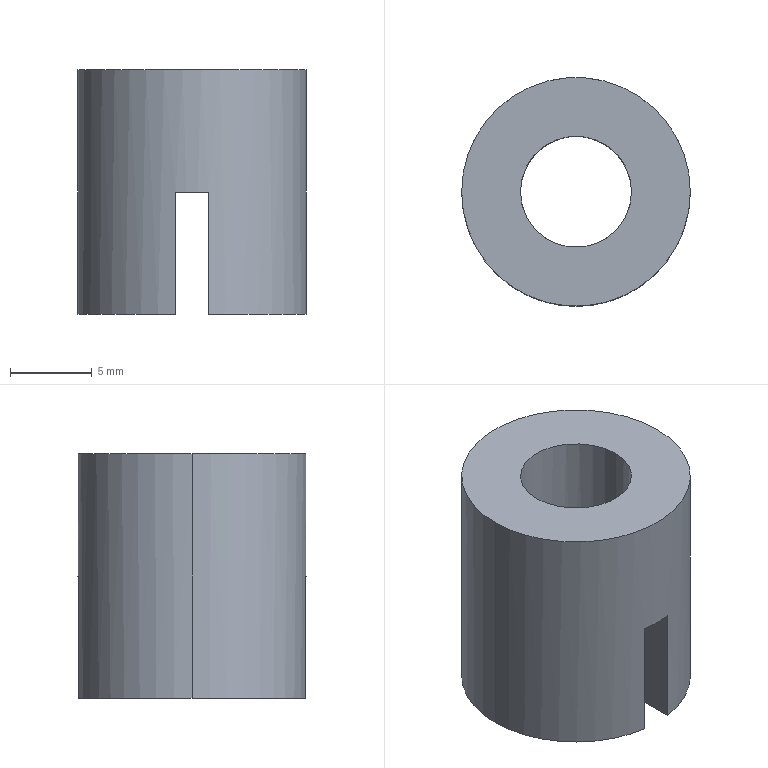Part | NX | features BREP 1 | 1 solid | 13 faces | box 14 x 14 x 15 mm | volume 1656 mm3 | plane 9 | cylinder 4 | commonest cylinder face diameters 6.8 x2 14 x2
STEP:
#1=CARTESIAN_POINT('',(3.4,0.,15.));
#2=VERTEX_POINT('',#1);
#3=CARTESIAN_POINT('',(-3.4,0.,15.));
#4=VERTEX_POINT('',#3);
#5=CARTESIAN_POINT('',(0.,0.,15.));
#6=DIRECTION('',(0.,0.,-1.));
#7=DIRECTION('',(-1.,0.,0.));
#8=AXIS2_PLACEMENT_3D('',#5,#6,#7);
#9=CIRCLE('',#8,3.4);
#10=EDGE_CURVE('',#2,#4,#9,.T.);
#11=ORIENTED_EDGE('',*,*,#10,.F.);
#12=CARTESIAN_POINT('',(3.4,0.,0.));
#13=VERTEX_POINT('',#12);
#14=CARTESIAN_POINT('',(3.4,0.,0.));
#15=DIRECTION('',(0.,0.,-1.));
#16=VECTOR('',#15,1000.);
#17=LINE('',#14,#16);
#18=EDGE_CURVE('',#2,#13,#17,.T.);
#19=ORIENTED_EDGE('',*,*,#18,.T.);
#20=CARTESIAN_POINT('',(1.,-3.25,0.));
#21=VERTEX_POINT('',#20);
#22=CARTESIAN_POINT('',(0.,0.,0.));
#23=DIRECTION('',(0.,0.,-1.));
#24=DIRECTION('',(-1.,0.,0.));
#25=AXIS2_PLACEMENT_3D('',#22,#23,#24);
#26=CIRCLE('',#25,3.4);
#27=EDGE_CURVE('',#13,#21,#26,.T.);
#28=ORIENTED_EDGE('',*,*,#27,.T.);
#29=CARTESIAN_POINT('',(1.,-3.25,7.5));
#30=VERTEX_POINT('',#29);
#31=CARTESIAN_POINT('',(1.,-3.25,0.));
#32=DIRECTION('',(0.,0.,1.));
#33=VECTOR('',#32,1000.);
#34=LINE('',#31,#33);
#35=EDGE_CURVE('',#21,#30,#34,.T.);
#36=ORIENTED_EDGE('',*,*,#35,.T.);
#37=CARTESIAN_POINT('',(-1.,-3.25,7.5));
#38=VERTEX_POINT('',#37);
#39=CARTESIAN_POINT('',(0.,0.,7.5));
#40=DIRECTION('',(0.,0.,-1.));
#41=DIRECTION('',(1.,0.,0.));
#42=AXIS2_PLACEMENT_3D('',#39,#40,#41);
#43=CIRCLE('',#42,3.4);
#44=EDGE_CURVE('',#30,#38,#43,.T.);
#45=ORIENTED_EDGE('',*,*,#44,.T.);
#46=CARTESIAN_POINT('',(-1.,-3.25,0.));
#47=VERTEX_POINT('',#46);
#48=CARTESIAN_POINT('',(-1.,-3.25,0.));
#49=DIRECTION('',(0.,0.,-1.));
#50=VECTOR('',#49,1000.);
#51=LINE('',#48,#50);
#52=EDGE_CURVE('',#38,#47,#51,.T.);
#53=ORIENTED_EDGE('',*,*,#52,.T.);
#54=CARTESIAN_POINT('',(-3.4,0.,0.));
#55=VERTEX_POINT('',#54);
#56=CARTESIAN_POINT('',(0.,0.,0.));
#57=DIRECTION('',(0.,0.,-1.));
#58=DIRECTION('',(-1.,0.,0.));
#59=AXIS2_PLACEMENT_3D('',#56,#57,#58);
#60=CIRCLE('',#59,3.4);
#61=EDGE_CURVE('',#47,#55,#60,.T.);
#62=ORIENTED_EDGE('',*,*,#61,.T.);
#63=CARTESIAN_POINT('',(-3.4,0.,0.));
#64=DIRECTION('',(0.,0.,-1.));
#65=VECTOR('',#64,1000.);
#66=LINE('',#63,#65);
#67=EDGE_CURVE('',#4,#55,#66,.T.);
#68=ORIENTED_EDGE('',*,*,#67,.F.);
#69=EDGE_LOOP('',(#11,#19,#28,#36,#45,#53,#62,#68));
#70=FACE_BOUND('',#69,.T.);
#71=CARTESIAN_POINT('',(0.,0.,0.));
#72=DIRECTION('',(0.,0.,-1.));
#73=DIRECTION('',(-1.,0.,0.));
#74=AXIS2_PLACEMENT_3D('',#71,#72,#73);
#75=CYLINDRICAL_SURFACE('',#74,3.4);
#76=ADVANCED_FACE('',(#70),#75,.F.);
#77=CARTESIAN_POINT('',(7.,0.,15.));
#78=VERTEX_POINT('',#77);
#79=CARTESIAN_POINT('',(-7.,0.,15.));
#80=VERTEX_POINT('',#79);
#81=CARTESIAN_POINT('',(0.,0.,15.));
#82=DIRECTION('',(0.,0.,1.));
#83=DIRECTION('',(1.,0.,0.));
#84=AXIS2_PLACEMENT_3D('',#81,#82,#83);
#85=CIRCLE('',#84,7.);
#86=EDGE_CURVE('',#78,#80,#85,.T.);
#87=ORIENTED_EDGE('',*,*,#86,.F.);
#88=CARTESIAN_POINT('',(7.,0.,0.));
#89=VERTEX_POINT('',#88);
#90=CARTESIAN_POINT('',(7.,0.,15.));
#91=DIRECTION('',(0.,0.,-1.));
#92=VECTOR('',#91,1000.);
#93=LINE('',#90,#92);
#94=EDGE_CURVE('',#78,#89,#93,.T.);
#95=ORIENTED_EDGE('',*,*,#94,.T.);
#96=CARTESIAN_POINT('',(1.,6.928,0.));
#97=VERTEX_POINT('',#96);
#98=CARTESIAN_POINT('',(0.,0.,0.));
#99=DIRECTION('',(0.,0.,1.));
#100=DIRECTION('',(1.,0.,0.));
#101=AXIS2_PLACEMENT_3D('',#98,#99,#100);
#102=CIRCLE('',#101,7.);
#103=EDGE_CURVE('',#89,#97,#102,.T.);
#104=ORIENTED_EDGE('',*,*,#103,.T.);
#105=CARTESIAN_POINT('',(1.,6.928,7.5));
#106=VERTEX_POINT('',#105);
#107=CARTESIAN_POINT('',(1.,6.928,15.));
#108=DIRECTION('',(0.,0.,1.));
#109=VECTOR('',#108,1000.);
#110=LINE('',#107,#109);
#111=EDGE_CURVE('',#97,#106,#110,.T.);
#112=ORIENTED_EDGE('',*,*,#111,.T.);
#113=CARTESIAN_POINT('',(-1.,6.928,7.5));
#114=VERTEX_POINT('',#113);
#115=CARTESIAN_POINT('',(0.,0.,7.5));
#116=DIRECTION('',(0.,0.,1.));
#117=DIRECTION('',(1.,0.,0.));
#118=AXIS2_PLACEMENT_3D('',#115,#116,#117);
#119=CIRCLE('',#118,7.);
#120=EDGE_CURVE('',#106,#114,#119,.T.);
#121=ORIENTED_EDGE('',*,*,#120,.T.);
#122=CARTESIAN_POINT('',(-1.,6.928,0.));
#123=VERTEX_POINT('',#122);
#124=CARTESIAN_POINT('',(-1.,6.928,15.));
#125=DIRECTION('',(0.,0.,-1.));
#126=VECTOR('',#125,1000.);
#127=LINE('',#124,#126);
#128=EDGE_CURVE('',#114,#123,#127,.T.);
#129=ORIENTED_EDGE('',*,*,#128,.T.);
#130=CARTESIAN_POINT('',(-7.,0.,0.));
#131=VERTEX_POINT('',#130);
#132=CARTESIAN_POINT('',(0.,0.,0.));
#133=DIRECTION('',(0.,0.,1.));
#134=DIRECTION('',(1.,0.,0.));
#135=AXIS2_PLACEMENT_3D('',#132,#133,#134);
#136=CIRCLE('',#135,7.);
#137=EDGE_CURVE('',#123,#131,#136,.T.);
#138=ORIENTED_EDGE('',*,*,#137,.T.);
#139=CARTESIAN_POINT('',(-7.,0.,15.));
#140=DIRECTION('',(0.,0.,-1.));
#141=VECTOR('',#140,1000.);
#142=LINE('',#139,#141);
#143=EDGE_CURVE('',#80,#131,#142,.T.);
#144=ORIENTED_EDGE('',*,*,#143,.F.);
#145=EDGE_LOOP('',(#87,#95,#104,#112,#121,#129,#138,#144));
#146=FACE_BOUND('',#145,.T.);
#147=CARTESIAN_POINT('',(0.,0.,15.));
#148=DIRECTION('',(0.,0.,-1.));
#149=DIRECTION('',(-1.,0.,0.));
#150=AXIS2_PLACEMENT_3D('',#147,#148,#149);
#151=CYLINDRICAL_SURFACE('',#150,7.);
#152=ADVANCED_FACE('',(#146),#151,.T.);
#153=ORIENTED_EDGE('',*,*,#137,.F.);
#154=CARTESIAN_POINT('',(-1.,3.25,0.));
#155=VERTEX_POINT('',#154);
#156=CARTESIAN_POINT('',(-1.,-7.,0.));
#157=DIRECTION('',(0.,1.,0.));
#158=VECTOR('',#157,1000.);
#159=LINE('',#156,#158);
#160=EDGE_CURVE('',#155,#123,#159,.T.);
#161=ORIENTED_EDGE('',*,*,#160,.F.);
#162=CARTESIAN_POINT('',(0.,0.,0.));
#163=DIRECTION('',(0.,0.,-1.));
#164=DIRECTION('',(-1.,0.,0.));
#165=AXIS2_PLACEMENT_3D('',#162,#163,#164);
#166=CIRCLE('',#165,3.4);
#167=EDGE_CURVE('',#55,#155,#166,.T.);
#168=ORIENTED_EDGE('',*,*,#167,.F.);
#169=ORIENTED_EDGE('',*,*,#61,.F.);
#170=CARTESIAN_POINT('',(-1.,-6.928,0.));
#171=VERTEX_POINT('',#170);
#172=CARTESIAN_POINT('',(-1.,-7.,0.));
#173=DIRECTION('',(0.,1.,0.));
#174=VECTOR('',#173,1000.);
#175=LINE('',#172,#174);
#176=EDGE_CURVE('',#171,#47,#175,.T.);
#177=ORIENTED_EDGE('',*,*,#176,.F.);
#178=CARTESIAN_POINT('',(0.,0.,0.));
#179=DIRECTION('',(0.,0.,1.));
#180=DIRECTION('',(1.,0.,0.));
#181=AXIS2_PLACEMENT_3D('',#178,#179,#180);
#182=CIRCLE('',#181,7.);
#183=EDGE_CURVE('',#131,#171,#182,.T.);
#184=ORIENTED_EDGE('',*,*,#183,.F.);
#185=EDGE_LOOP('',(#153,#161,#168,#169,#177,#184));
#186=FACE_BOUND('',#185,.T.);
#187=CARTESIAN_POINT('',(0.,0.,0.));
#188=DIRECTION('',(0.,0.,1.));
#189=DIRECTION('',(1.,0.,0.));
#190=AXIS2_PLACEMENT_3D('',#187,#188,#189);
#191=PLANE('',#190);
#192=ADVANCED_FACE('',(#186),#191,.F.);
#193=ORIENTED_EDGE('',*,*,#94,.F.);
#194=CARTESIAN_POINT('',(0.,0.,15.));
#195=DIRECTION('',(0.,0.,1.));
#196=DIRECTION('',(1.,0.,0.));
#197=AXIS2_PLACEMENT_3D('',#194,#195,#196);
#198=CIRCLE('',#197,7.);
#199=EDGE_CURVE('',#80,#78,#198,.T.);
#200=ORIENTED_EDGE('',*,*,#199,.F.);
#201=ORIENTED_EDGE('',*,*,#143,.T.);
#202=ORIENTED_EDGE('',*,*,#183,.T.);
#203=CARTESIAN_POINT('',(-1.,-6.928,7.5));
#204=VERTEX_POINT('',#203);
#205=CARTESIAN_POINT('',(-1.,-6.928,15.));
#206=DIRECTION('',(0.,0.,1.));
#207=VECTOR('',#206,1000.);
#208=LINE('',#205,#207);
#209=EDGE_CURVE('',#171,#204,#208,.T.);
#210=ORIENTED_EDGE('',*,*,#209,.T.);
#211=CARTESIAN_POINT('',(1.,-6.928,7.5));
#212=VERTEX_POINT('',#211);
#213=CARTESIAN_POINT('',(0.,0.,7.5));
#214=DIRECTION('',(0.,0.,1.));
#215=DIRECTION('',(1.,0.,0.));
#216=AXIS2_PLACEMENT_3D('',#213,#214,#215);
#217=CIRCLE('',#216,7.);
#218=EDGE_CURVE('',#204,#212,#217,.T.);
#219=ORIENTED_EDGE('',*,*,#218,.T.);
#220=CARTESIAN_POINT('',(1.,-6.928,0.));
#221=VERTEX_POINT('',#220);
#222=CARTESIAN_POINT('',(1.,-6.928,15.));
#223=DIRECTION('',(0.,0.,-1.));
#224=VECTOR('',#223,1000.);
#225=LINE('',#222,#224);
#226=EDGE_CURVE('',#212,#221,#225,.T.);
#227=ORIENTED_EDGE('',*,*,#226,.T.);
#228=CARTESIAN_POINT('',(0.,0.,0.));
#229=DIRECTION('',(0.,0.,1.));
#230=DIRECTION('',(1.,0.,0.));
#231=AXIS2_PLACEMENT_3D('',#228,#229,#230);
#232=CIRCLE('',#231,7.);
#233=EDGE_CURVE('',#221,#89,#232,.T.);
#234=ORIENTED_EDGE('',*,*,#233,.T.);
#235=EDGE_LOOP('',(#193,#200,#201,#202,#210,#219,#227,#234));
#236=FACE_BOUND('',#235,.T.);
#237=CARTESIAN_POINT('',(0.,0.,15.));
#238=DIRECTION('',(0.,0.,-1.));
#239=DIRECTION('',(-1.,0.,0.));
#240=AXIS2_PLACEMENT_3D('',#237,#238,#239);
#241=CYLINDRICAL_SURFACE('',#240,7.);
#242=ADVANCED_FACE('',(#236),#241,.T.);
#243=ORIENTED_EDGE('',*,*,#199,.T.);
#244=ORIENTED_EDGE('',*,*,#86,.T.);
#245=EDGE_LOOP('',(#243,#244));
#246=FACE_BOUND('',#245,.T.);
#247=CARTESIAN_POINT('',(0.,0.,15.));
#248=DIRECTION('',(0.,0.,-1.));
#249=DIRECTION('',(-1.,0.,0.));
#250=AXIS2_PLACEMENT_3D('',#247,#248,#249);
#251=CIRCLE('',#250,3.4);
#252=EDGE_CURVE('',#4,#2,#251,.T.);
#253=ORIENTED_EDGE('',*,*,#252,.T.);
#254=ORIENTED_EDGE('',*,*,#10,.T.);
#255=EDGE_LOOP('',(#253,#254));
#256=FACE_BOUND('',#255,.T.);
#257=CARTESIAN_POINT('',(0.,0.,15.));
#258=DIRECTION('',(0.,0.,1.));
#259=DIRECTION('',(1.,0.,0.));
#260=AXIS2_PLACEMENT_3D('',#257,#258,#259);
#261=PLANE('',#260);
#262=ADVANCED_FACE('',(#246,#256),#261,.T.);
#263=ORIENTED_EDGE('',*,*,#233,.F.);
#264=CARTESIAN_POINT('',(1.,-7.,0.));
#265=DIRECTION('',(0.,-1.,0.));
#266=VECTOR('',#265,1000.);
#267=LINE('',#264,#266);
#268=EDGE_CURVE('',#21,#221,#267,.T.);
#269=ORIENTED_EDGE('',*,*,#268,.F.);
#270=ORIENTED_EDGE('',*,*,#27,.F.);
#271=CARTESIAN_POINT('',(1.,3.25,0.));
#272=VERTEX_POINT('',#271);
#273=CARTESIAN_POINT('',(0.,0.,0.));
#274=DIRECTION('',(0.,0.,-1.));
#275=DIRECTION('',(-1.,0.,0.));
#276=AXIS2_PLACEMENT_3D('',#273,#274,#275);
#277=CIRCLE('',#276,3.4);
#278=EDGE_CURVE('',#272,#13,#277,.T.);
#279=ORIENTED_EDGE('',*,*,#278,.F.);
#280=CARTESIAN_POINT('',(1.,-7.,0.));
#281=DIRECTION('',(0.,-1.,0.));
#282=VECTOR('',#281,1000.);
#283=LINE('',#280,#282);
#284=EDGE_CURVE('',#97,#272,#283,.T.);
#285=ORIENTED_EDGE('',*,*,#284,.F.);
#286=ORIENTED_EDGE('',*,*,#103,.F.);
#287=EDGE_LOOP('',(#263,#269,#270,#279,#285,#286));
#288=FACE_BOUND('',#287,.T.);
#289=CARTESIAN_POINT('',(0.,0.,0.));
#290=DIRECTION('',(0.,0.,1.));
#291=DIRECTION('',(1.,0.,0.));
#292=AXIS2_PLACEMENT_3D('',#289,#290,#291);
#293=PLANE('',#292);
#294=ADVANCED_FACE('',(#288),#293,.F.);
#295=ORIENTED_EDGE('',*,*,#18,.F.);
#296=ORIENTED_EDGE('',*,*,#252,.F.);
#297=ORIENTED_EDGE('',*,*,#67,.T.);
#298=ORIENTED_EDGE('',*,*,#167,.T.);
#299=CARTESIAN_POINT('',(-1.,3.25,7.5));
#300=VERTEX_POINT('',#299);
#301=CARTESIAN_POINT('',(-1.,3.25,0.));
#302=DIRECTION('',(0.,0.,1.));
#303=VECTOR('',#302,1000.);
#304=LINE('',#301,#303);
#305=EDGE_CURVE('',#155,#300,#304,.T.);
#306=ORIENTED_EDGE('',*,*,#305,.T.);
#307=CARTESIAN_POINT('',(1.,3.25,7.5));
#308=VERTEX_POINT('',#307);
#309=CARTESIAN_POINT('',(0.,0.,7.5));
#310=DIRECTION('',(0.,0.,-1.));
#311=DIRECTION('',(1.,0.,0.));
#312=AXIS2_PLACEMENT_3D('',#309,#310,#311);
#313=CIRCLE('',#312,3.4);
#314=EDGE_CURVE('',#300,#308,#313,.T.);
#315=ORIENTED_EDGE('',*,*,#314,.T.);
#316=CARTESIAN_POINT('',(1.,3.25,0.));
#317=DIRECTION('',(0.,0.,-1.));
#318=VECTOR('',#317,1000.);
#319=LINE('',#316,#318);
#320=EDGE_CURVE('',#308,#272,#319,.T.);
#321=ORIENTED_EDGE('',*,*,#320,.T.);
#322=ORIENTED_EDGE('',*,*,#278,.T.);
#323=EDGE_LOOP('',(#295,#296,#297,#298,#306,#315,#321,#322));
#324=FACE_BOUND('',#323,.T.);
#325=CARTESIAN_POINT('',(0.,0.,0.));
#326=DIRECTION('',(0.,0.,-1.));
#327=DIRECTION('',(-1.,0.,0.));
#328=AXIS2_PLACEMENT_3D('',#325,#326,#327);
#329=CYLINDRICAL_SURFACE('',#328,3.4);
#330=ADVANCED_FACE('',(#324),#329,.F.);
#331=CARTESIAN_POINT('',(1.,-7.,7.5));
#332=DIRECTION('',(0.,-1.,0.));
#333=VECTOR('',#332,1000.);
#334=LINE('',#331,#333);
#335=EDGE_CURVE('',#106,#308,#334,.T.);
#336=ORIENTED_EDGE('',*,*,#335,.T.);
#337=ORIENTED_EDGE('',*,*,#314,.F.);
#338=CARTESIAN_POINT('',(-1.,-7.,7.5));
#339=DIRECTION('',(0.,1.,0.));
#340=VECTOR('',#339,1000.);
#341=LINE('',#338,#340);
#342=EDGE_CURVE('',#300,#114,#341,.T.);
#343=ORIENTED_EDGE('',*,*,#342,.T.);
#344=ORIENTED_EDGE('',*,*,#120,.F.);
#345=EDGE_LOOP('',(#336,#337,#343,#344));
#346=FACE_BOUND('',#345,.T.);
#347=CARTESIAN_POINT('',(0.,0.,7.5));
#348=DIRECTION('',(0.,0.,1.));
#349=DIRECTION('',(1.,0.,0.));
#350=AXIS2_PLACEMENT_3D('',#347,#348,#349);
#351=PLANE('',#350);
#352=ADVANCED_FACE('',(#346),#351,.F.);
#353=ORIENTED_EDGE('',*,*,#284,.T.);
#354=ORIENTED_EDGE('',*,*,#320,.F.);
#355=ORIENTED_EDGE('',*,*,#335,.F.);
#356=ORIENTED_EDGE('',*,*,#111,.F.);
#357=EDGE_LOOP('',(#353,#354,#355,#356));
#358=FACE_BOUND('',#357,.T.);
#359=CARTESIAN_POINT('',(1.,-7.,7.5));
#360=DIRECTION('',(1.,0.,0.));
#361=DIRECTION('',(0.,1.,0.));
#362=AXIS2_PLACEMENT_3D('',#359,#360,#361);
#363=PLANE('',#362);
#364=ADVANCED_FACE('',(#358),#363,.F.);
#365=ORIENTED_EDGE('',*,*,#342,.F.);
#366=ORIENTED_EDGE('',*,*,#305,.F.);
#367=ORIENTED_EDGE('',*,*,#160,.T.);
#368=ORIENTED_EDGE('',*,*,#128,.F.);
#369=EDGE_LOOP('',(#365,#366,#367,#368));
#370=FACE_BOUND('',#369,.T.);
#371=CARTESIAN_POINT('',(-1.,-7.,7.5));
#372=DIRECTION('',(-1.,0.,0.));
#373=DIRECTION('',(0.,0.,1.));
#374=AXIS2_PLACEMENT_3D('',#371,#372,#373);
#375=PLANE('',#374);
#376=ADVANCED_FACE('',(#370),#375,.F.);
#377=ORIENTED_EDGE('',*,*,#176,.T.);
#378=ORIENTED_EDGE('',*,*,#52,.F.);
#379=CARTESIAN_POINT('',(-1.,-7.,7.5));
#380=DIRECTION('',(0.,1.,0.));
#381=VECTOR('',#380,1000.);
#382=LINE('',#379,#381);
#383=EDGE_CURVE('',#204,#38,#382,.T.);
#384=ORIENTED_EDGE('',*,*,#383,.F.);
#385=ORIENTED_EDGE('',*,*,#209,.F.);
#386=EDGE_LOOP('',(#377,#378,#384,#385));
#387=FACE_BOUND('',#386,.T.);
#388=CARTESIAN_POINT('',(-1.,-7.,7.5));
#389=DIRECTION('',(-1.,0.,0.));
#390=DIRECTION('',(0.,0.,1.));
#391=AXIS2_PLACEMENT_3D('',#388,#389,#390);
#392=PLANE('',#391);
#393=ADVANCED_FACE('',(#387),#392,.F.);
#394=CARTESIAN_POINT('',(1.,-7.,7.5));
#395=DIRECTION('',(0.,-1.,0.));
#396=VECTOR('',#395,1000.);
#397=LINE('',#394,#396);
#398=EDGE_CURVE('',#30,#212,#397,.T.);
#399=ORIENTED_EDGE('',*,*,#398,.F.);
#400=ORIENTED_EDGE('',*,*,#35,.F.);
#401=ORIENTED_EDGE('',*,*,#268,.T.);
#402=ORIENTED_EDGE('',*,*,#226,.F.);
#403=EDGE_LOOP('',(#399,#400,#401,#402));
#404=FACE_BOUND('',#403,.T.);
#405=CARTESIAN_POINT('',(1.,-7.,7.5));
#406=DIRECTION('',(1.,0.,0.));
#407=DIRECTION('',(0.,1.,0.));
#408=AXIS2_PLACEMENT_3D('',#405,#406,#407);
#409=PLANE('',#408);
#410=ADVANCED_FACE('',(#404),#409,.F.);
#411=ORIENTED_EDGE('',*,*,#383,.T.);
#412=ORIENTED_EDGE('',*,*,#44,.F.);
#413=ORIENTED_EDGE('',*,*,#398,.T.);
#414=ORIENTED_EDGE('',*,*,#218,.F.);
#415=EDGE_LOOP('',(#411,#412,#413,#414));
#416=FACE_BOUND('',#415,.T.);
#417=CARTESIAN_POINT('',(0.,0.,7.5));
#418=DIRECTION('',(0.,0.,1.));
#419=DIRECTION('',(1.,0.,0.));
#420=AXIS2_PLACEMENT_3D('',#417,#418,#419);
#421=PLANE('',#420);
#422=ADVANCED_FACE('',(#416),#421,.F.);
#423=CLOSED_SHELL('',(#76,#152,#192,#242,#262,#294,#330,#352,#364,#376,#393,#410,#422));
#424=MANIFOLD_SOLID_BREP('',#423);
#425=(LENGTH_UNIT()NAMED_UNIT(*)SI_UNIT(.MILLI.,.METRE.));
#426=UNCERTAINTY_MEASURE_WITH_UNIT(LENGTH_MEASURE(0.00001),#425,'','');
#427=(NAMED_UNIT(*)PLANE_ANGLE_UNIT()SI_UNIT($,.RADIAN.));
#428=(NAMED_UNIT(*)SI_UNIT($,.STERADIAN.)SOLID_ANGLE_UNIT());
#429=(GEOMETRIC_REPRESENTATION_CONTEXT(3)GLOBAL_UNCERTAINTY_ASSIGNED_CONTEXT((#426))GLOBAL_UNIT_ASSIGNED_CONTEXT((#425,#427,#428))REPRESENTATION_CONTEXT('',''));
#430=ADVANCED_BREP_SHAPE_REPRESENTATION('',(#424),#429);